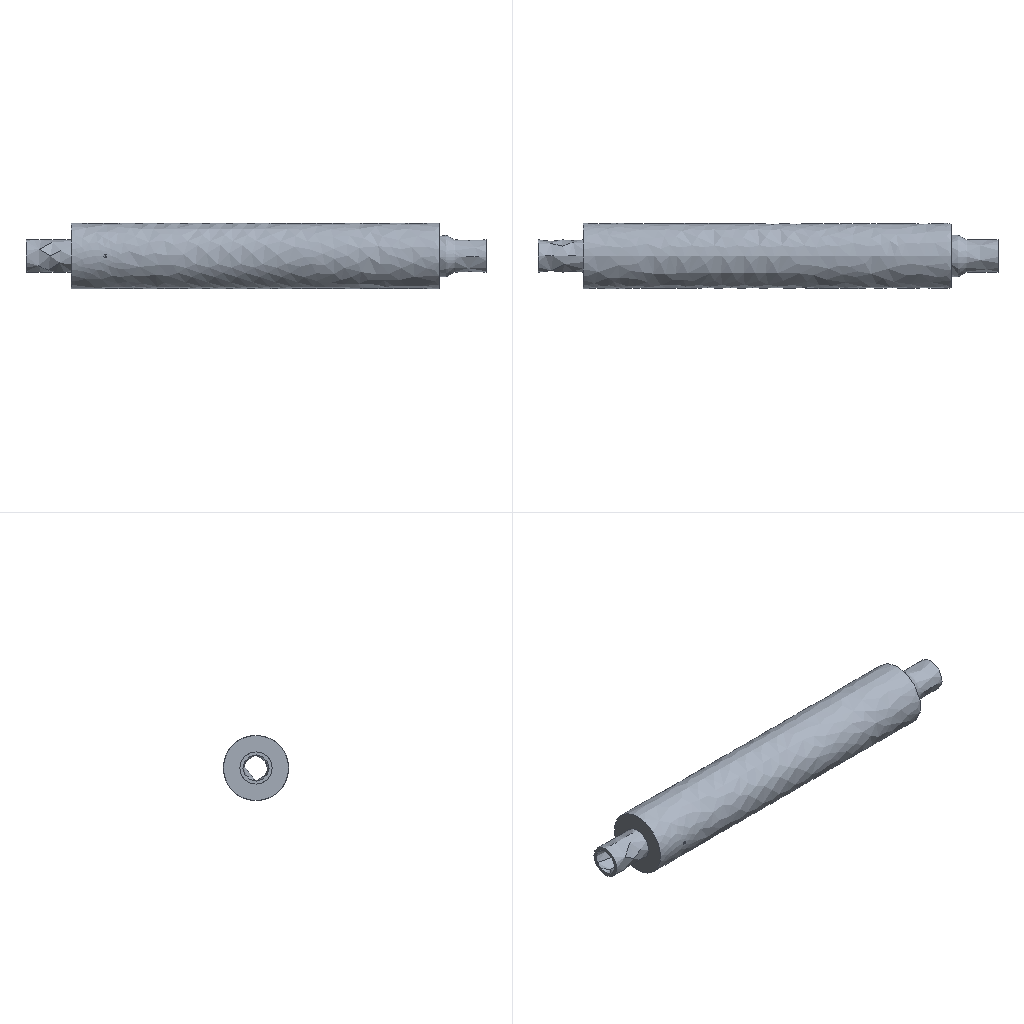Simulation study | ansys workbench
Set-up summary:
category,name,step,type,value,unit,region
solver,ansys_workbench
units,mm-N-s-tonne (MPa),,stated,"/units,MPA"
analysis,LS1,,static
load_step,LS1,LS1,static,nsubst=1; time=1
mesh,nodes,,,178790
mesh,elements,,,94488
element_type,SOLID187,,,91263
element_type,SURF154,,,1236
element_type,TARGE170,,,816
element_type,CONTA174,,,816
element_type,SOLID186,,,357
material,Structural Steel,,E,200000,tonne s^-2 mm^-1
material,Structural Steel,,nu,0.3
material,Structural Steel,,density,7.85e-09,tonne mm^-3
material,Structural Steel,,conductivity,60.5,tonne mm s^-3 C^-1
material,Structural Steel,,specific_heat,4.34e+08,mm^2 s^-2 C^-1
material,Structural Steel,,cte,1.2e-05,C^-1
material,Structural Steel,,permeability,10000
material,Structural Steel,,resistivity,0.00017,ohm mm
load,"Define Pressure Using Surface Effect Elements ""__""",LS1,pressure,3,,SURF154 #17
load,Component For All Non-Zero UX Displacements,LS1,body load temp,-296,,_CM76
bc,Fixed Supports,model,fixed,[dofs=ALL],,_FIXEDSU
bc,Set Displacements,LS1,prescribed ux,50 [dofs=UX],,_CM68UX_XP
contact,Contact Region,,bonded (always),element=CONTA174
contact,Contact Region 2,,bonded (always),element=CONTA174
contact,Contact Region 3,,bonded (always),element=CONTA174
contact,Contact Region 4,,bonded (always),element=CONTA174
contact,Contact Region 5,,bonded (always),element=CONTA174
named_set,_FIXEDSU,,node,663
named_set,_CM68UX_XP,,node,84
Ansys APDL input file, long lists of numbers shortened:
/batch
/config,noeldb,1     ! force off writing results to database
*get,_wallstrt,active,,time,wall
! ANSYS input file written by Workbench version 2022 R1
! File used for geometry attach:
/title,wbnew--____ (B5)
! ****** Begin Custom Load Command Snippet ******
/COM, ACT Extensions:
/COM,     LSDYNA, 2021.1
/COM,
! ****** End   Custom Load Command Snippet ******
*DIM,_wb_ProjectScratch_dir,string,248
_wb_ProjectScratch_dir(1) = ''
*DIM,_wb_SolverFiles_dir,string,248
_wb_SolverFiles_dir(1) = ''
*DIM,_wb_userfiles_dir,string,248
_wb_userfiles_dir(1) = ''
/com,--- Data in consistent NMM units. See Solving Units in the help system for more information.
/units,MPA
/nopr
/wb,file,start              !  signify a WB generated input file
/prep7
! Turn off shape checking because checks already performed inside WB mesher.
! See help system for more information.
SHPP,OFF,,NOWARN
/nolist
etcon,set             ! allow ANSYS to choose best KEYOP's for 180x elements, resets any applicable keyopt to MAPDL defaults
/com,*********** Nodes for the whole assembly ***********
nblock,3,,196669
(1i9,3e20.9e3)
        1     2.439032187E+02     4.925080413E+01     8.165016973E+01
! (178789 more lines like these left out)
-1
/wb,elem,start            !  set before creation of elements
/com,*********** Elements for Body 1 "-01__1|__1" ***********
et,1,187
eblock,19,solid,,1107
(19i9)
        1        1        1        1        0        0        0        0       10        0     4348    10627    10812    10639    10887    11978    12059    11973    11980
! (2213 more lines like these left out)
-1
/com,*********** Elements for Body 2 "-02___|__1" ***********
et,2,187
eblock,19,solid,,84562
(19i9)
        2        2        2        2        0        0        0        0       10        0     7059    24217    38159    38158    31511   115439   174111   115438   115437
! (169123 more lines like these left out)
-1
/com,*********** Elements for Body 3 "-04___|__1" ***********
et,3,186
keyo,3,2,1          ! set full integration on SOLID186
eblock,19,solid,,357
(19i9)
        3        3        3        3        0        0        0        0       20        0      223      870     1164     1163      871      874     1169     1168      872
! (713 more lines like these left out)
-1
/com,*********** Elements for Body 4 "-05__2|__1" ***********
et,4,187
eblock,19,solid,,1604
(19i9)
        4        4        4        4        0        0        0        0       10        0     5455    12805    12812    13178    13341    13510    13578    13513    13518
! (3207 more lines like these left out)
-1
/com,*********** Elements for Body 5 "-06__|__1" ***********
et,5,187
eblock,19,solid,,222
(19i9)
        5        5        5        5        0        0        0        0       10        0        1       40       73       51       85      359      408      357      362
! (443 more lines like these left out)
-1
/com,*********** Elements for Body 6 "-03___|__-__1" ***********
et,6,187
eblock,19,solid,,3768
(19i9)
        6        6        6        6        0        0        0        0       10        0      580     2806     3128     2813     4097     4172     4208     4171     4174
! (7535 more lines like these left out)
-1
/wb,elem,end               !  done creating elements
/com,*********** Send User Defined Coordinate System(s) ***********
csys,0
toffst,273.15,  ! Temperature offset from absolute zero
/com,*********** Set Reference Temperature ***********
tref,22.
/wb,mat,start              !  starting to send materials
/com,*********** Send Materials ***********
Temperature = 'TEMP' ! Temperature
MP,DENS,1,7.85e-09,	! tonne mm^-3
MP,ALPX,1,1.2e-05,	! C^-1
MP,C,1,434000000,	! mm^2 s^-2 C^-1
MP,KXX,1,60.5,	! tonne mm s^-3 C^-1
MP,RSVX,1,0.00017,	! ohm mm
MP,EX,1,200000,	! tonne s^-2 mm^-1
MP,NUXY,1,0.3,
MP,MURX,1,10000,
Temperature = 'TEMP' ! Temperature
MP,DENS,2,7.85e-09,	! tonne mm^-3
MP,ALPX,2,1.2e-05,	! C^-1
MP,C,2,434000000,	! mm^2 s^-2 C^-1
MP,KXX,2,60.5,	! tonne mm s^-3 C^-1
MP,RSVX,2,0.00017,	! ohm mm
MP,EX,2,200000,	! tonne s^-2 mm^-1
MP,NUXY,2,0.3,
MP,MURX,2,10000,
Temperature = 'TEMP' ! Temperature
MP,DENS,3,7.85e-09,	! tonne mm^-3
MP,ALPX,3,1.2e-05,	! C^-1
MP,C,3,434000000,	! mm^2 s^-2 C^-1
MP,KXX,3,60.5,	! tonne mm s^-3 C^-1
MP,RSVX,3,0.00017,	! ohm mm
MP,EX,3,200000,	! tonne s^-2 mm^-1
MP,NUXY,3,0.3,
MP,MURX,3,10000,
Temperature = 'TEMP' ! Temperature
MP,DENS,4,7.85e-09,	! tonne mm^-3
MP,ALPX,4,1.2e-05,	! C^-1
MP,C,4,434000000,	! mm^2 s^-2 C^-1
MP,KXX,4,60.5,	! tonne mm s^-3 C^-1
MP,RSVX,4,0.00017,	! ohm mm
MP,EX,4,200000,	! tonne s^-2 mm^-1
MP,NUXY,4,0.3,
MP,MURX,4,10000,
Temperature = 'TEMP' ! Temperature
MP,DENS,5,7.85e-09,	! tonne mm^-3
MP,ALPX,5,1.2e-05,	! C^-1
MP,C,5,434000000,	! mm^2 s^-2 C^-1
MP,KXX,5,60.5,	! tonne mm s^-3 C^-1
MP,RSVX,5,0.00017,	! ohm mm
MP,EX,5,200000,	! tonne s^-2 mm^-1
MP,NUXY,5,0.3,
MP,MURX,5,10000,
Temperature = 'TEMP' ! Temperature
MP,DENS,6,7.85e-09,	! tonne mm^-3
MP,ALPX,6,1.2e-05,	! C^-1
MP,C,6,434000000,	! mm^2 s^-2 C^-1
MP,KXX,6,60.5,	! tonne mm s^-3 C^-1
MP,RSVX,6,0.00017,	! ohm mm
MP,EX,6,200000,	! tonne s^-2 mm^-1
MP,NUXY,6,0.3,
MP,MURX,6,10000,
/wb,mat,end                !  done sending materials
!************************* Model Summary ********************
!-01__1|__1,	结构钢,	matid,	1
!-02___|__1,	结构钢,	matid,	2
!-04___|__1,	结构钢,	matid,	3
!-05__2|__1,	结构钢,	matid,	4
!-06__|__1,	结构钢,	matid,	5
!-03___|__-__1,	结构钢,	matid,	6
!************************* End Model Summary ********************
! get the diagonal of the bounding box. Needed later for other things
*get,_xmin,node,,mnloc,x
*get,_ymin,node,,mnloc,y
*get,_zmin,node,,mnloc,z
*get,_xmax,node,,mxloc,x
*get,_ymax,node,,mxloc,y
*get,_zmax,node,,mxloc,z
_ASMDIAG=(_xmax-_xmin)*(_xmax-_xmin)+(_ymax-_ymin)*(_ymax-_ymin)+(_zmax-_zmin)*(_zmax-_zmin)
_ASMDIAG=SQRT(_ASMDIAG)
/wb,contact,start          !  starting to send contact
/com,*********** Create Contact "接触区域" ***********
/com,            Real Constant Set For Above Contact Is 8 & 7
*set,tid,8
*set,cid,7
r,tid
r,cid
et,tid,170
et,cid,174
eblock,10,,,36
(15i9)
   146707        8        8        8        0    10635    10639    10812    10812    12030    12059    10812    12035
! (35 more lines like these left out)
-1
eblock,10,,,36
(15i9)
   146743        7        7        7        0    10635    10639    10812    10812    12030    12059    10812    12035
! (35 more lines like these left out)
-1
eblock,10,,,134
(15i9)
   146779        7        8        7        0    23502    17399    38692    38692    56111    56118    38692   109964
! (133 more lines like these left out)
-1
eblock,10,,,134
(15i9)
   146913        8        7        8        0    23502    17399    38692    38692    56111    56118    38692   109964
! (133 more lines like these left out)
-1
keyo,cid,8,2               ! auto create asymmetric contact (from Program Controlled setting)
keyo,cid,10,0              ! adjust contact stiffness each NR iteration (from Program Controlled setting)
keyo,cid,12,5              ! bonded always
keyo,cid,18,1              ! small sliding turned on by application
keyo,cid,2,0               ! augmented Lagrange (from Program Controlled setting)
keyo,cid,4,0               ! on Gauss point (from Program Controlled setting)
keyo,cid,9,1               ! ignore initial gaps/penetration
keyo,cid,7,0               ! No Prediction
rmod,tid,3,10.      ! FKN
rmod,tid,5,0.       ! ICONT
rmod,tid,6,0.       ! PINB
rmod,tid,10,0.      ! CNOF
rmod,tid,12,0.      ! FKT
rmod,tid,36,41      ! WB DSID
rmod,cid,3,10.      ! FKN
rmod,cid,5,0.       ! ICONT
rmod,cid,6,0.       ! PINB
rmod,cid,10,0.      ! CNOF
rmod,cid,12,0.      ! FKT
rmod,cid,36,41      ! WB DSID
/com,*********** Create Contact "接触区域 2" ***********
/com,            Real Constant Set For Above Contact Is 10 & 9
*set,tid,10
*set,cid,9
r,tid
r,cid
et,tid,170
et,cid,174
eblock,10,,,32
(15i9)
   147047       10       10       10        0    10496    10821    10649    10649    10986    12120    10649    10983
! (31 more lines like these left out)
-1
eblock,10,,,32
(15i9)
   147079        9        9        9        0    10496    10821    10649    10649    10986    12120    10649    10983
! (31 more lines like these left out)
-1
eblock,10,,,17
(15i9)
   147111        9       10        9        0      575      574      560      560     1310     1271      560     1272
! (16 more lines like these left out)
-1
eblock,10,,,17
(15i9)
   147128       10        9       10        0      575      574      560      560     1310     1271      560     1272
! (16 more lines like these left out)
-1
keyo,cid,8,2               ! auto create asymmetric contact (from Program Controlled setting)
keyo,cid,10,0              ! adjust contact stiffness each NR iteration (from Program Controlled setting)
keyo,cid,12,5              ! bonded always
keyo,cid,18,1              ! small sliding turned on by application
keyo,cid,2,0               ! augmented Lagrange (from Program Controlled setting)
keyo,cid,4,0               ! on Gauss point (from Program Controlled setting)
keyo,cid,9,1               ! ignore initial gaps/penetration
keyo,cid,7,0               ! No Prediction
rmod,tid,3,10.      ! FKN
rmod,tid,5,0.       ! ICONT
rmod,tid,6,0.       ! PINB
rmod,tid,10,0.      ! CNOF
rmod,tid,12,0.      ! FKT
rmod,tid,36,44      ! WB DSID
rmod,cid,3,10.      ! FKN
rmod,cid,5,0.       ! ICONT
rmod,cid,6,0.       ! PINB
rmod,cid,10,0.      ! CNOF
rmod,cid,12,0.      ! FKT
rmod,cid,36,44      ! WB DSID
/com,*********** Create Contact "接触区域 3" ***********
/com,            Real Constant Set For Above Contact Is 12 & 11
*set,tid,12
*set,cid,11
r,tid
r,cid
et,tid,170
et,cid,174
eblock,10,,,112
(15i9)
   147145       12       12       12        0    10542    10549    10717    10717    11354    11432    10717    11359
! (111 more lines like these left out)
-1
eblock,10,,,112
(15i9)
   147257       11       11       11        0    10542    10549    10717    10717    11354    11432    10717    11359
! (111 more lines like these left out)
-1
eblock,10,,,126
(15i9)
   147369       11       12       11        0     3105     2815     3012     3012     4223     4220     3012     5562
! (125 more lines like these left out)
-1
eblock,10,,,126
(15i9)
   147495       12       11       12        0     3105     2815     3012     3012     4223     4220     3012     5562
! (125 more lines like these left out)
-1
keyo,cid,8,2               ! auto create asymmetric contact (from Program Controlled setting)
keyo,cid,10,0              ! adjust contact stiffness each NR iteration (from Program Controlled setting)
keyo,cid,12,5              ! bonded always
keyo,cid,18,1              ! small sliding turned on by application
keyo,cid,2,0               ! augmented Lagrange (from Program Controlled setting)
keyo,cid,4,0               ! on Gauss point (from Program Controlled setting)
keyo,cid,9,1               ! ignore initial gaps/penetration
keyo,cid,7,0               ! No Prediction
rmod,tid,3,10.      ! FKN
rmod,tid,5,0.       ! ICONT
rmod,tid,6,0.       ! PINB
rmod,tid,10,0.      ! CNOF
rmod,tid,12,0.      ! FKT
rmod,tid,36,47      ! WB DSID
rmod,cid,3,10.      ! FKN
rmod,cid,5,0.       ! ICONT
rmod,cid,6,0.       ! PINB
rmod,cid,10,0.      ! CNOF
rmod,cid,12,0.      ! FKT
rmod,cid,36,47      ! WB DSID
/com,*********** Create Contact "接触区域 4" ***********
/com,            Real Constant Set For Above Contact Is 14 & 13
*set,tid,14
*set,cid,13
r,tid
r,cid
et,tid,170
et,cid,174
eblock,10,,,131
(15i9)
   147621       14       14       14        0    41738    23219    23208    23208   107694   107607    23208   107616
! (130 more lines like these left out)
-1
eblock,10,,,131
(15i9)
   147752       13       13       13        0    41738    23219    23208    23208   107694   107607    23208   107616
! (130 more lines like these left out)
-1
eblock,10,,,32
(15i9)
   147883       13       14       13        0    12913    12914    12931    12931    14355    14366    12931    14357
! (31 more lines like these left out)
-1
eblock,10,,,32
(15i9)
   147915       14       13       14        0    12913    12914    12931    12931    14355    14366    12931    14357
! (31 more lines like these left out)
-1
keyo,cid,8,2               ! auto create asymmetric contact (from Program Controlled setting)
keyo,cid,10,0              ! adjust contact stiffness each NR iteration (from Program Controlled setting)
keyo,cid,12,5              ! bonded always
keyo,cid,18,1              ! small sliding turned on by application
keyo,cid,2,0               ! augmented Lagrange (from Program Controlled setting)
keyo,cid,4,0               ! on Gauss point (from Program Controlled setting)
keyo,cid,9,1               ! ignore initial gaps/penetration
keyo,cid,7,0               ! No Prediction
rmod,tid,3,10.      ! FKN
rmod,tid,5,0.       ! ICONT
rmod,tid,6,0.       ! PINB
rmod,tid,10,0.      ! CNOF
rmod,tid,12,0.      ! FKT
rmod,tid,36,50      ! WB DSID
rmod,cid,3,10.      ! FKN
rmod,cid,5,0.       ! ICONT
rmod,cid,6,0.       ! PINB
rmod,cid,10,0.      ! CNOF
rmod,cid,12,0.      ! FKT
rmod,cid,36,50      ! WB DSID
/com,*********** Create Contact "接触区域 5" ***********
/com,            Real Constant Set For Above Contact Is 16 & 15
*set,tid,16
*set,cid,15
r,tid
r,cid
et,tid,170
et,cid,174
eblock,10,,,98
(15i9)
   147947       16       16       16        0       30       37       90       90      307      344       90      309
! (97 more lines like these left out)
-1
eblock,10,,,98
(15i9)
   148045       15       15       15        0       30       37       90       90      307      344       90      309
! (97 more lines like these left out)
-1
eblock,10,,,98
(15i9)
   148143       15       16       15        0     2846     3119     3035     3035     4487     5700     3035     4484
! (97 more lines like these left out)
-1
eblock,10,,,98
(15i9)
   148241       16       15       16        0     2846     3119     3035     3035     4487     5700     3035     4484
! (97 more lines like these left out)
-1
keyo,cid,8,2               ! auto create asymmetric contact (from Program Controlled setting)
keyo,cid,10,0              ! adjust contact stiffness each NR iteration (from Program Controlled setting)
keyo,cid,12,5              ! bonded always
keyo,cid,18,1              ! small sliding turned on by application
keyo,cid,2,0               ! augmented Lagrange (from Program Controlled setting)
keyo,cid,4,0               ! on Gauss point (from Program Controlled setting)
keyo,cid,9,1               ! ignore initial gaps/penetration
keyo,cid,7,0               ! No Prediction
rmod,tid,3,10.      ! FKN
rmod,tid,5,0.       ! ICONT
rmod,tid,6,0.       ! PINB
rmod,tid,10,0.      ! CNOF
rmod,tid,12,0.      ! FKT
rmod,tid,36,53      ! WB DSID
rmod,cid,3,10.      ! FKN
rmod,cid,5,0.       ! ICONT
rmod,cid,6,0.       ! PINB
rmod,cid,10,0.      ! CNOF
rmod,cid,12,0.      ! FKT
rmod,cid,36,53      ! WB DSID
nsel,all
esel,all
/wb,contact,end            !  done creating contacts
/golist
/wb,load,start             !  starting to send loads
/com,*********** Fixed Supports ***********
CMBLOCK,_FIXEDSU,NODE,      663
(8i10)
         1         2         3         4         5         6        29        30
! (82 more lines like these left out)
cmsel,s,_FIXEDSU
d,all,all
nsel,all
/com,*********** Define Pressure Using Surface Effect Elements "__" ***********
et,17,154
eblock,10,,,1236
(15i9)
   148339       17       17       17        0     2972     2971     3126     3126     5362     5363     3126     5368
! (1235 more lines like these left out)
-1
esel,s,type,,17
keyop,17,7,0                ! Use deformed area for application of load
esel,all
/com,*********** Define Body Force Temperature ***********
esel,none
esel,a,type,,1
esel,a,type,,2,6
cm,_CM76,elem
esel,all
esel,all
/gst,on,on
fini
*get,_numnode,node,0,count
*get,_numelem,elem,0,count
*get, _MAXELEMNUM, elem, 0, NUM, MAX
*get, _MAXNODENUM, node, 0, NUM, MAX
*get, _MAXELEMTYPE, etyp, 0, NUM, MAX
*get, _MAXREALCONST, real, 0, NUM, MAX
/go
/wb,load,end               !  done creating loads
/com,--- Number of total nodes = %_numnode%
/com,--- Number of contact elements = 2868
/com,--- Number of spring elements = 0
/com,--- Number of bearing elements = 0
/com,--- Number of solid elements = 91620
/com,--- Number of condensed parts = 0
/com,--- Number of total elements = %_numelem%
*get,_wallbsol,active,,time,wall
/com,****************************************************************************
/com,*************************    SOLUTION       ********************************
/com,****************************************************************************
/solu
antype,0                   ! static analysis
_thickRatio=  0     ! Ratio of thick parts in the model
eqsl,sparse,,,,,1
cntr,print,1               ! print out contact info and also make no initial contact an error
dmpoption,emat,no             ! Don't combine emat file for DANSYS
dmpoption,esav,no             ! Don't combine esav file for DANSYS
nldiag,cont,iter           ! print out contact info each equilibrium iteration
rescontrol,,none                 ! Do not keep any restart files
/com,****************************************************
/com,******************* SOLVE FOR LS 1 OF 1 ****************
esel,s,type,,17
nsle
sf,all,pres,3.
nsel,all
esel,all
/com,*** Set Displacements ***
CMBLOCK,_CM68UX_XP,NODE,       84
(8i10)
     12871     12874     12875     12876     12877     12884     12887     12888
! (10 more lines like these left out)
cmsel,s,_CM68UX_XP
d,all,ux,50.
nsel,all
/com,*** Component For All Non-Zero UX Displacements ***
cmsel,s,_CM68ux_xp
cm,_DISPNONZEROUX,NODE
nsel,all
esel,all
/nopr
cmsel,s,_CM76
nsle
bf,all,temp,-296.
nsel,all
esel,all
/gopr
nsub,1,1,1
time,1.
outres,erase
outres,all,none
outres,nsol,all,
outres,rsol,all
outres,eangl,all
outres,etmp,all
outres,veng,all
outres,strs,all,
outres,epel,all,
outres,eppl,all,
outres,epth,all,
outres,cont,all,
! *********** WB SOLVE COMMAND ***********
! check interactive state
*get,ANSINTER_,active,,int
*if,ANSINTER_,ne,0,then
/eof
*endif
solve
/com *************** Write FE CONNECTORS *********
CEWRITE,file,ce,,INTE
/com,****************************************************
/com,*************** FINISHED SOLVE FOR LS 1 *************
*get,_wallasol,active,,time,wall
/nopr
*get,_numnode,node,0,count
*get,_numelem,elem,0,count
*get, _MAXELEMNUM, elem, 0, NUM, MAX
*get, _MAXNODENUM, node, 0, NUM, MAX,,,INTERNAL
*get, _MAXELEMTYPE, etyp, 0, NUM, MAX
*get, _MAXREALCONST, real, 0, NUM, MAX
/gopr
/post1
xmlo,ENCODING,ISO-8859-1
xmlo,parm
/xml,parm,xml
fini
/gopr
*get,_walldone,active,,time,wall
_preptime=(_wallbsol-_wallstrt)*3600
_solvtime=(_wallasol-_wallbsol)*3600
_posttime=(_walldone-_wallasol)*3600
_totaltim=(_walldone-_wallstrt)*3600
*get,_dlbratio,active,0,solu,dlbr
*get,_combtime,active,0,solu,comb
*get,_ssmode,active,0,solu,ssmm
*get,_ndofs,active,0,solu,ndof
*get,_sol_end_time,active,0,set,time
*if,_sol_end_time,eq,1.,then
/fclean				!clean distributed files
*endif
/com,--- Total number of nodes = %_numnode%
/com,--- Total number of elements = %_numelem%
/com,--- Element load balance ratio = %_dlbratio%
/com,--- Time to combine distributed files = %_combtime%
/com,--- Sparse memory mode = %_ssmode%
/com,--- Number of DOF = %_ndofs%
/wb,file,end               ! done with WB generated input
Results summary:
result,analyses[0].index,,,1
result,analyses[0].system,,,SYS
result,analyses[0].deck,,,deck.dat
result,analyses[0].solve_status,,,completed
result,analyses[0].analysis_type,,,static
result,analyses[0].physics,,,mechanical
result,analyses[0].unit_system,,,"NMM: mm, ton, N, s, mV, mA, degC"
result,analyses[0].n_sets,,,1
result,analyses[0].load_steps[0].set,set=1,,1
result,analyses[0].load_steps[0].time_or_freq,set=1,,1
result,analyses[0].load_steps[0].max_displacement_magnitude,set=1,,50.37
result,analyses[0].load_steps[0].max_von_mises_nodal,set=1,,9958.47
result,analyses[0].load_steps[0].reaction_force_sum_xyz[1],set=1,,-0.000355
result,analyses[0].load_steps[0].reaction_force_sum_xyz[2],set=1,,0.0002441
result,analyses[0].load_steps[0].reaction_force_sum_xyz[3],set=1,,-0.0002299